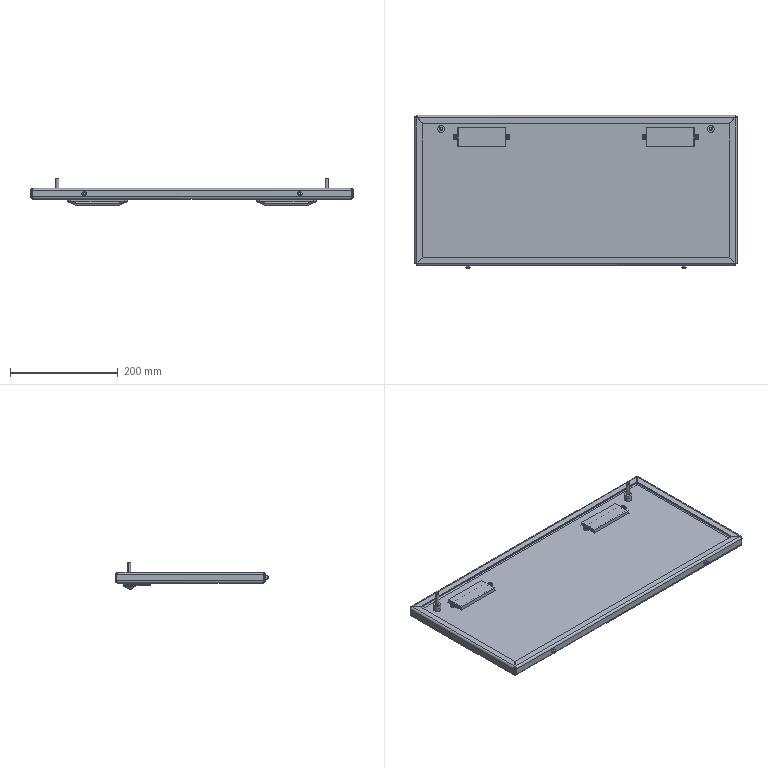Part | NX | features BREP 3 | 5 solids | 422 faces | box 598 x 284 x 51.5 mm | volume 479261 mm3 | plane 216 | cylinder 166 | spline 16 | torus 12 | cone 12 | commonest cylinder face diameters 6 x20 10 x20 4 x16 7 x14 8 x12 8.6 x12